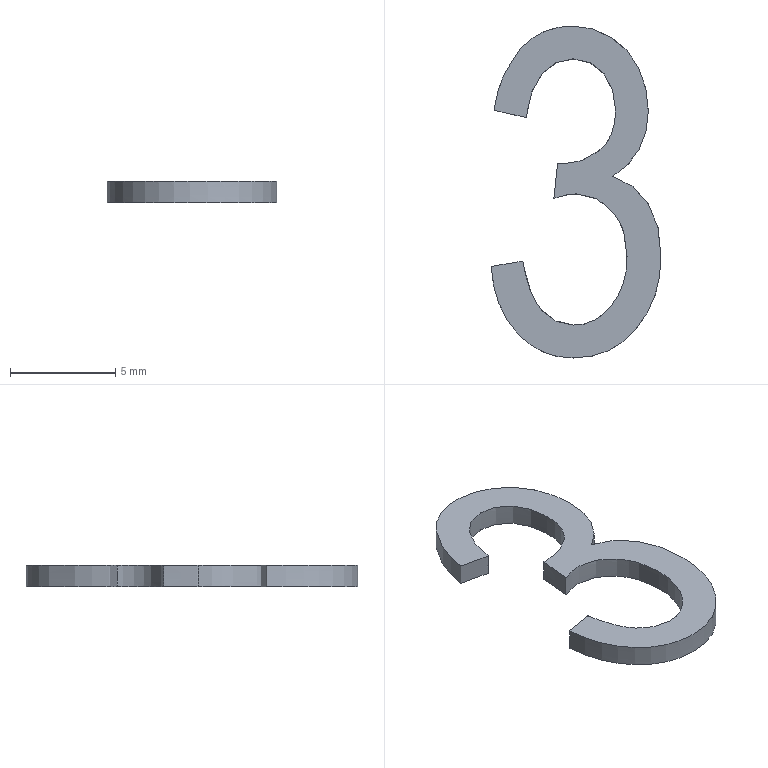Part | STEP file | lll_id962_x_t | 1 solid | 3 faces | box 8.074 x 15.771 x 1 mm | volume 33.504 mm3 | plane 2 | other 1